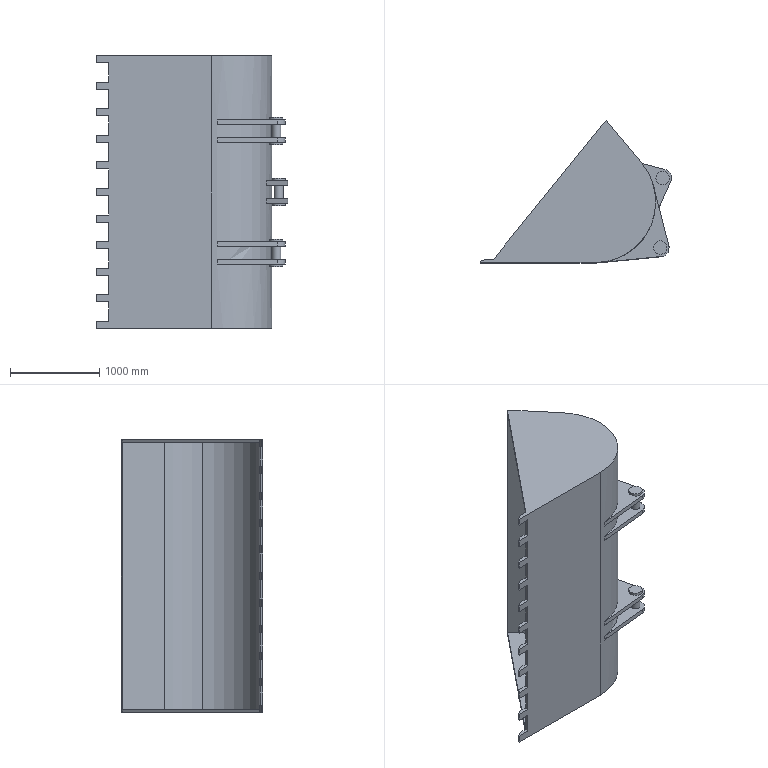Part | SolidWorks | features ICE 11, Extrusion 1, LPattern 1, MirrorPattern 1 | 1 solid | 148 faces | box 2144 x 1589 x 3060 mm | volume 438244984 mm3 | plane 115 | cylinder 33 | commonest cylinder face diameters 150 x12 200 x9 100 x6 1360 x4 1300 x2